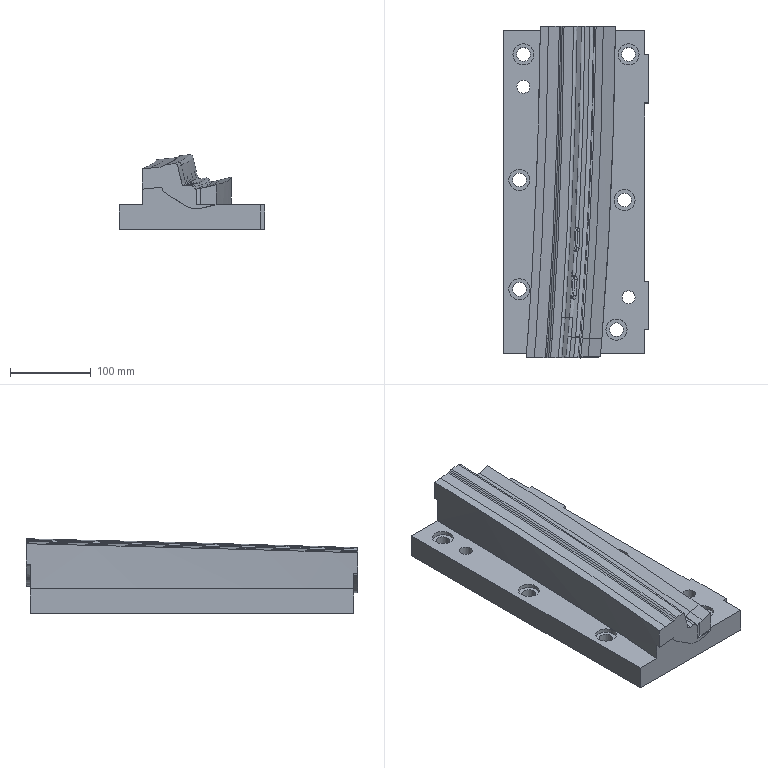Part | NX | features solid 2 | 1 solid | 110 faces | box 180 x 410.001 x 91.937 mm | volume 3545726 mm3 | spline 65 | plane 28 | cylinder 17 | commonest cylinder face diameters 17 x6 26 x6 16 x2 25 x2 20 x1